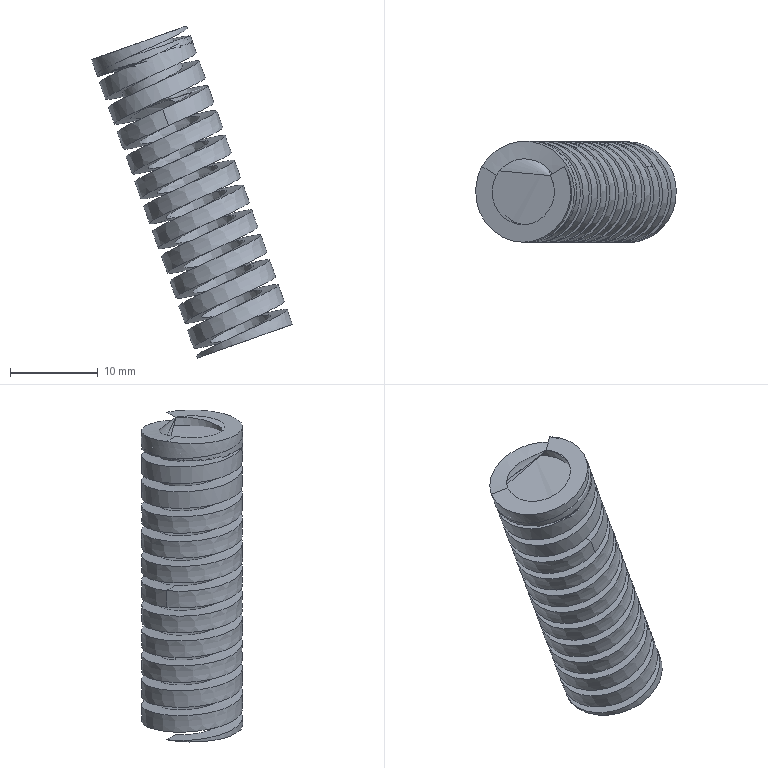Part | STEP file | SPRING_id686_x_t | 1 solid | 19 faces | box 22.825 x 11.499 x 37.765 mm | volume 1937 mm3 | spline 17 | plane 2